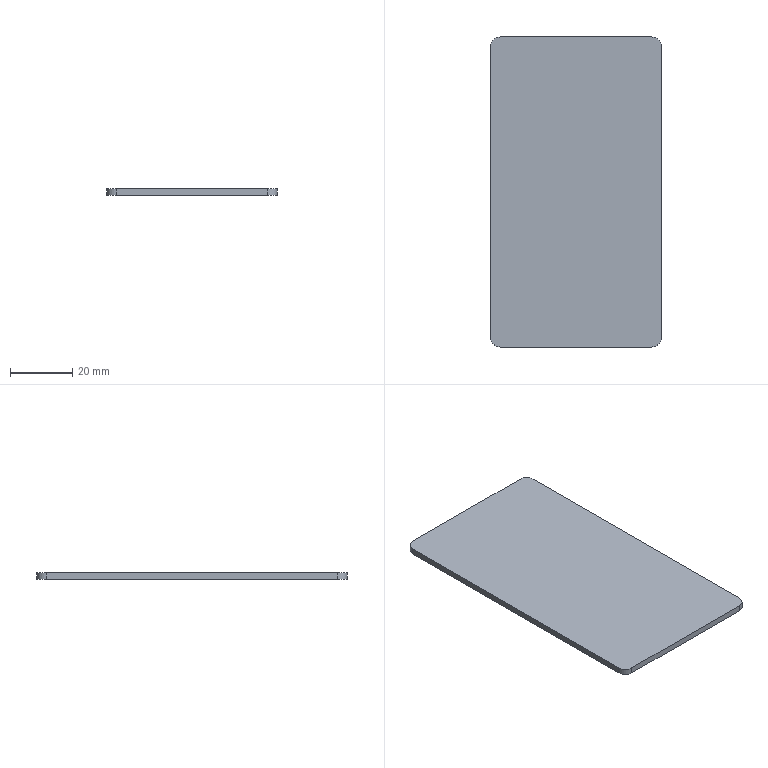Part | STEP file | E3-踢脚Plate支Plate | 1 solid | 10 faces | box 55 x 100 x 2 mm | volume 10985 mm3 | plane 6 | cylinder 4 | commonest cylinder face diameters 6 x4
STEP:
#1=CARTESIAN_POINT('',(0.,0.,0.));
#2=DIRECTION('',(0.,0.,1.));
#3=DIRECTION('',(1.,0.,0.));
#4=AXIS2_PLACEMENT_3D('',#1,#2,#3);
#5=CARTESIAN_POINT('',(27.5,-47.,-2.));
#6=VERTEX_POINT('',#5);
#7=CARTESIAN_POINT('',(27.5,47.,-2.));
#8=VERTEX_POINT('',#7);
#9=CARTESIAN_POINT('',(27.5,50.,-2.));
#10=DIRECTION('',(0.,1.,0.));
#11=VECTOR('',#10,1.);
#12=LINE('',#9,#11);
#13=CARTESIAN_POINT('',(27.5,50.,-2.));
#14=DIRECTION('',(-1.,0.,0.));
#15=DIRECTION('',(0.,0.,-1.));
#16=AXIS2_PLACEMENT_3D('',#13,#14,#15);
#17=PLANE('',#16);
#18=CARTESIAN_POINT('',(0.,0.));
#19=DIRECTION('',(0.,-1.));
#20=VECTOR('',#19,1.);
#21=LINE('',#18,#20);
#22=(GEOMETRIC_REPRESENTATION_CONTEXT(2)PARAMETRIC_REPRESENTATION_CONTEXT()REPRESENTATION_CONTEXT('',''));
#23=DEFINITIONAL_REPRESENTATION('',(#21),#22);
#24=PCURVE('',#17,#23);
#25=CARTESIAN_POINT('',(0.,0.,-2.));
#26=DIRECTION('',(0.,0.,-1.));
#27=DIRECTION('',(1.,0.,0.));
#28=AXIS2_PLACEMENT_3D('',#25,#26,#27);
#29=PLANE('',#28);
#30=CARTESIAN_POINT('',(27.5,-50.));
#31=DIRECTION('',(0.,-1.));
#32=VECTOR('',#31,1.);
#33=LINE('',#30,#32);
#34=(GEOMETRIC_REPRESENTATION_CONTEXT(2)PARAMETRIC_REPRESENTATION_CONTEXT()REPRESENTATION_CONTEXT('',''));
#35=DEFINITIONAL_REPRESENTATION('',(#33),#34);
#36=PCURVE('',#29,#35);
#37=SURFACE_CURVE('',#12,(#24,#36),.PCURVE_S1.);
#38=EDGE_CURVE('',#6,#8,#37,.T.);
#39=ORIENTED_EDGE('',*,*,#38,.T.);
#40=CARTESIAN_POINT('',(27.5,47.,0.));
#41=VERTEX_POINT('',#40);
#42=CARTESIAN_POINT('',(27.5,47.,-2.));
#43=DIRECTION('',(0.,0.,-1.));
#44=VECTOR('',#43,1.);
#45=LINE('',#42,#44);
#46=CARTESIAN_POINT('',(0.,3.));
#47=DIRECTION('',(1.,0.));
#48=VECTOR('',#47,1.);
#49=LINE('',#46,#48);
#50=(GEOMETRIC_REPRESENTATION_CONTEXT(2)PARAMETRIC_REPRESENTATION_CONTEXT()REPRESENTATION_CONTEXT('',''));
#51=DEFINITIONAL_REPRESENTATION('',(#49),#50);
#52=PCURVE('',#17,#51);
#53=CARTESIAN_POINT('',(24.5,47.,-2.));
#54=DIRECTION('',(0.,0.,1.));
#55=DIRECTION('',(-1.,0.,0.));
#56=AXIS2_PLACEMENT_3D('',#53,#54,#55);
#57=CYLINDRICAL_SURFACE('',#56,3.);
#58=CARTESIAN_POINT('',(3.142,0.));
#59=DIRECTION('',(0.,-1.));
#60=VECTOR('',#59,1.);
#61=LINE('',#58,#60);
#62=(GEOMETRIC_REPRESENTATION_CONTEXT(2)PARAMETRIC_REPRESENTATION_CONTEXT()REPRESENTATION_CONTEXT('',''));
#63=DEFINITIONAL_REPRESENTATION('',(#61),#62);
#64=PCURVE('',#57,#63);
#65=SURFACE_CURVE('',#45,(#52,#64),.PCURVE_S1.);
#66=EDGE_CURVE('',#41,#8,#65,.T.);
#67=ORIENTED_EDGE('',*,*,#66,.F.);
#68=CARTESIAN_POINT('',(27.5,-47.,0.));
#69=VERTEX_POINT('',#68);
#70=CARTESIAN_POINT('',(27.5,50.,0.));
#71=DIRECTION('',(0.,1.,0.));
#72=VECTOR('',#71,1.);
#73=LINE('',#70,#72);
#74=CARTESIAN_POINT('',(-2.,0.));
#75=DIRECTION('',(0.,-1.));
#76=VECTOR('',#75,1.);
#77=LINE('',#74,#76);
#78=(GEOMETRIC_REPRESENTATION_CONTEXT(2)PARAMETRIC_REPRESENTATION_CONTEXT()REPRESENTATION_CONTEXT('',''));
#79=DEFINITIONAL_REPRESENTATION('',(#77),#78);
#80=PCURVE('',#17,#79);
#81=CARTESIAN_POINT('',(0.,0.,0.));
#82=DIRECTION('',(0.,0.,-1.));
#83=DIRECTION('',(1.,0.,0.));
#84=AXIS2_PLACEMENT_3D('',#81,#82,#83);
#85=PLANE('',#84);
#86=CARTESIAN_POINT('',(27.5,-50.));
#87=DIRECTION('',(0.,-1.));
#88=VECTOR('',#87,1.);
#89=LINE('',#86,#88);
#90=(GEOMETRIC_REPRESENTATION_CONTEXT(2)PARAMETRIC_REPRESENTATION_CONTEXT()REPRESENTATION_CONTEXT('',''));
#91=DEFINITIONAL_REPRESENTATION('',(#89),#90);
#92=PCURVE('',#85,#91);
#93=SURFACE_CURVE('',#73,(#80,#92),.PCURVE_S1.);
#94=EDGE_CURVE('',#69,#41,#93,.T.);
#95=ORIENTED_EDGE('',*,*,#94,.F.);
#96=CARTESIAN_POINT('',(27.5,-47.,-2.));
#97=DIRECTION('',(0.,0.,1.));
#98=VECTOR('',#97,1.);
#99=LINE('',#96,#98);
#100=CARTESIAN_POINT('',(0.,97.));
#101=DIRECTION('',(-1.,0.));
#102=VECTOR('',#101,1.);
#103=LINE('',#100,#102);
#104=(GEOMETRIC_REPRESENTATION_CONTEXT(2)PARAMETRIC_REPRESENTATION_CONTEXT()REPRESENTATION_CONTEXT('',''));
#105=DEFINITIONAL_REPRESENTATION('',(#103),#104);
#106=PCURVE('',#17,#105);
#107=CARTESIAN_POINT('',(24.5,-47.,-2.));
#108=DIRECTION('',(0.,0.,1.));
#109=DIRECTION('',(-1.,0.,0.));
#110=AXIS2_PLACEMENT_3D('',#107,#108,#109);
#111=CYLINDRICAL_SURFACE('',#110,3.);
#112=CARTESIAN_POINT('',(3.142,0.));
#113=DIRECTION('',(0.,1.));
#114=VECTOR('',#113,1.);
#115=LINE('',#112,#114);
#116=(GEOMETRIC_REPRESENTATION_CONTEXT(2)PARAMETRIC_REPRESENTATION_CONTEXT()REPRESENTATION_CONTEXT('',''));
#117=DEFINITIONAL_REPRESENTATION('',(#115),#116);
#118=PCURVE('',#111,#117);
#119=SURFACE_CURVE('',#99,(#106,#118),.PCURVE_S1.);
#120=EDGE_CURVE('',#6,#69,#119,.T.);
#121=ORIENTED_EDGE('',*,*,#120,.F.);
#122=EDGE_LOOP('',(#39,#67,#95,#121));
#123=FACE_BOUND('',#122,.T.);
#124=ADVANCED_FACE('',(#123),#17,.F.);
#125=CARTESIAN_POINT('',(24.5,50.,-2.));
#126=VERTEX_POINT('',#125);
#127=CARTESIAN_POINT('',(-24.5,50.,-2.));
#128=VERTEX_POINT('',#127);
#129=CARTESIAN_POINT('',(-27.5,50.,-2.));
#130=DIRECTION('',(-1.,0.,0.));
#131=VECTOR('',#130,1.);
#132=LINE('',#129,#131);
#133=CARTESIAN_POINT('',(-27.5,50.,-2.));
#134=DIRECTION('',(0.,-1.,0.));
#135=DIRECTION('',(0.,0.,1.));
#136=AXIS2_PLACEMENT_3D('',#133,#134,#135);
#137=PLANE('',#136);
#138=CARTESIAN_POINT('',(0.,0.));
#139=DIRECTION('',(0.,1.));
#140=VECTOR('',#139,1.);
#141=LINE('',#138,#140);
#142=(GEOMETRIC_REPRESENTATION_CONTEXT(2)PARAMETRIC_REPRESENTATION_CONTEXT()REPRESENTATION_CONTEXT('',''));
#143=DEFINITIONAL_REPRESENTATION('',(#141),#142);
#144=PCURVE('',#137,#143);
#145=CARTESIAN_POINT('',(-27.5,-50.));
#146=DIRECTION('',(-1.,0.));
#147=VECTOR('',#146,1.);
#148=LINE('',#145,#147);
#149=(GEOMETRIC_REPRESENTATION_CONTEXT(2)PARAMETRIC_REPRESENTATION_CONTEXT()REPRESENTATION_CONTEXT('',''));
#150=DEFINITIONAL_REPRESENTATION('',(#148),#149);
#151=PCURVE('',#29,#150);
#152=SURFACE_CURVE('',#132,(#144,#151),.PCURVE_S1.);
#153=EDGE_CURVE('',#126,#128,#152,.T.);
#154=ORIENTED_EDGE('',*,*,#153,.T.);
#155=CARTESIAN_POINT('',(-24.5,50.,0.));
#156=VERTEX_POINT('',#155);
#157=CARTESIAN_POINT('',(-24.5,50.,-2.));
#158=DIRECTION('',(0.,0.,-1.));
#159=VECTOR('',#158,1.);
#160=LINE('',#157,#159);
#161=CARTESIAN_POINT('',(0.,-3.));
#162=DIRECTION('',(-1.,0.));
#163=VECTOR('',#162,1.);
#164=LINE('',#161,#163);
#165=(GEOMETRIC_REPRESENTATION_CONTEXT(2)PARAMETRIC_REPRESENTATION_CONTEXT()REPRESENTATION_CONTEXT('',''));
#166=DEFINITIONAL_REPRESENTATION('',(#164),#165);
#167=PCURVE('',#137,#166);
#168=CARTESIAN_POINT('',(-24.5,47.,-2.));
#169=DIRECTION('',(0.,0.,1.));
#170=DIRECTION('',(-1.,0.,0.));
#171=AXIS2_PLACEMENT_3D('',#168,#169,#170);
#172=CYLINDRICAL_SURFACE('',#171,3.);
#173=CARTESIAN_POINT('',(4.712,0.));
#174=DIRECTION('',(0.,-1.));
#175=VECTOR('',#174,1.);
#176=LINE('',#173,#175);
#177=(GEOMETRIC_REPRESENTATION_CONTEXT(2)PARAMETRIC_REPRESENTATION_CONTEXT()REPRESENTATION_CONTEXT('',''));
#178=DEFINITIONAL_REPRESENTATION('',(#176),#177);
#179=PCURVE('',#172,#178);
#180=SURFACE_CURVE('',#160,(#167,#179),.PCURVE_S1.);
#181=EDGE_CURVE('',#156,#128,#180,.T.);
#182=ORIENTED_EDGE('',*,*,#181,.F.);
#183=CARTESIAN_POINT('',(24.5,50.,0.));
#184=VERTEX_POINT('',#183);
#185=CARTESIAN_POINT('',(-27.5,50.,0.));
#186=DIRECTION('',(-1.,0.,0.));
#187=VECTOR('',#186,1.);
#188=LINE('',#185,#187);
#189=CARTESIAN_POINT('',(2.,0.));
#190=DIRECTION('',(0.,1.));
#191=VECTOR('',#190,1.);
#192=LINE('',#189,#191);
#193=(GEOMETRIC_REPRESENTATION_CONTEXT(2)PARAMETRIC_REPRESENTATION_CONTEXT()REPRESENTATION_CONTEXT('',''));
#194=DEFINITIONAL_REPRESENTATION('',(#192),#193);
#195=PCURVE('',#137,#194);
#196=CARTESIAN_POINT('',(-27.5,-50.));
#197=DIRECTION('',(-1.,0.));
#198=VECTOR('',#197,1.);
#199=LINE('',#196,#198);
#200=(GEOMETRIC_REPRESENTATION_CONTEXT(2)PARAMETRIC_REPRESENTATION_CONTEXT()REPRESENTATION_CONTEXT('',''));
#201=DEFINITIONAL_REPRESENTATION('',(#199),#200);
#202=PCURVE('',#85,#201);
#203=SURFACE_CURVE('',#188,(#195,#202),.PCURVE_S1.);
#204=EDGE_CURVE('',#184,#156,#203,.T.);
#205=ORIENTED_EDGE('',*,*,#204,.F.);
#206=CARTESIAN_POINT('',(24.5,50.,-2.));
#207=DIRECTION('',(0.,0.,1.));
#208=VECTOR('',#207,1.);
#209=LINE('',#206,#208);
#210=CARTESIAN_POINT('',(0.,-52.));
#211=DIRECTION('',(1.,0.));
#212=VECTOR('',#211,1.);
#213=LINE('',#210,#212);
#214=(GEOMETRIC_REPRESENTATION_CONTEXT(2)PARAMETRIC_REPRESENTATION_CONTEXT()REPRESENTATION_CONTEXT('',''));
#215=DEFINITIONAL_REPRESENTATION('',(#213),#214);
#216=PCURVE('',#137,#215);
#217=CARTESIAN_POINT('',(4.712,0.));
#218=DIRECTION('',(0.,1.));
#219=VECTOR('',#218,1.);
#220=LINE('',#217,#219);
#221=(GEOMETRIC_REPRESENTATION_CONTEXT(2)PARAMETRIC_REPRESENTATION_CONTEXT()REPRESENTATION_CONTEXT('',''));
#222=DEFINITIONAL_REPRESENTATION('',(#220),#221);
#223=PCURVE('',#57,#222);
#224=SURFACE_CURVE('',#209,(#216,#223),.PCURVE_S1.);
#225=EDGE_CURVE('',#126,#184,#224,.T.);
#226=ORIENTED_EDGE('',*,*,#225,.F.);
#227=EDGE_LOOP('',(#154,#182,#205,#226));
#228=FACE_BOUND('',#227,.T.);
#229=ADVANCED_FACE('',(#228),#137,.F.);
#230=CARTESIAN_POINT('',(-27.5,47.,0.));
#231=VERTEX_POINT('',#230);
#232=CARTESIAN_POINT('',(-27.5,-47.,0.));
#233=VERTEX_POINT('',#232);
#234=CARTESIAN_POINT('',(-27.5,50.,0.));
#235=DIRECTION('',(0.,-1.,0.));
#236=VECTOR('',#235,1.);
#237=LINE('',#234,#236);
#238=CARTESIAN_POINT('',(-27.5,50.,-2.));
#239=DIRECTION('',(1.,0.,0.));
#240=DIRECTION('',(0.,0.,1.));
#241=AXIS2_PLACEMENT_3D('',#238,#239,#240);
#242=PLANE('',#241);
#243=CARTESIAN_POINT('',(2.,0.));
#244=DIRECTION('',(0.,1.));
#245=VECTOR('',#244,1.);
#246=LINE('',#243,#245);
#247=(GEOMETRIC_REPRESENTATION_CONTEXT(2)PARAMETRIC_REPRESENTATION_CONTEXT()REPRESENTATION_CONTEXT('',''));
#248=DEFINITIONAL_REPRESENTATION('',(#246),#247);
#249=PCURVE('',#242,#248);
#250=CARTESIAN_POINT('',(-27.5,-50.));
#251=DIRECTION('',(0.,1.));
#252=VECTOR('',#251,1.);
#253=LINE('',#250,#252);
#254=(GEOMETRIC_REPRESENTATION_CONTEXT(2)PARAMETRIC_REPRESENTATION_CONTEXT()REPRESENTATION_CONTEXT('',''));
#255=DEFINITIONAL_REPRESENTATION('',(#253),#254);
#256=PCURVE('',#85,#255);
#257=SURFACE_CURVE('',#237,(#249,#256),.PCURVE_S1.);
#258=EDGE_CURVE('',#231,#233,#257,.T.);
#259=ORIENTED_EDGE('',*,*,#258,.F.);
#260=CARTESIAN_POINT('',(-27.5,47.,-2.));
#261=VERTEX_POINT('',#260);
#262=CARTESIAN_POINT('',(-27.5,47.,-2.));
#263=DIRECTION('',(0.,0.,1.));
#264=VECTOR('',#263,1.);
#265=LINE('',#262,#264);
#266=CARTESIAN_POINT('',(0.,3.));
#267=DIRECTION('',(1.,0.));
#268=VECTOR('',#267,1.);
#269=LINE('',#266,#268);
#270=(GEOMETRIC_REPRESENTATION_CONTEXT(2)PARAMETRIC_REPRESENTATION_CONTEXT()REPRESENTATION_CONTEXT('',''));
#271=DEFINITIONAL_REPRESENTATION('',(#269),#270);
#272=PCURVE('',#242,#271);
#273=CARTESIAN_POINT('',(6.283,0.));
#274=DIRECTION('',(0.,1.));
#275=VECTOR('',#274,1.);
#276=LINE('',#273,#275);
#277=(GEOMETRIC_REPRESENTATION_CONTEXT(2)PARAMETRIC_REPRESENTATION_CONTEXT()REPRESENTATION_CONTEXT('',''));
#278=DEFINITIONAL_REPRESENTATION('',(#276),#277);
#279=PCURVE('',#172,#278);
#280=SURFACE_CURVE('',#265,(#272,#279),.PCURVE_S1.);
#281=EDGE_CURVE('',#261,#231,#280,.T.);
#282=ORIENTED_EDGE('',*,*,#281,.F.);
#283=CARTESIAN_POINT('',(-27.5,-47.,-2.));
#284=VERTEX_POINT('',#283);
#285=CARTESIAN_POINT('',(-27.5,50.,-2.));
#286=DIRECTION('',(0.,-1.,0.));
#287=VECTOR('',#286,1.);
#288=LINE('',#285,#287);
#289=CARTESIAN_POINT('',(0.,0.));
#290=DIRECTION('',(0.,1.));
#291=VECTOR('',#290,1.);
#292=LINE('',#289,#291);
#293=(GEOMETRIC_REPRESENTATION_CONTEXT(2)PARAMETRIC_REPRESENTATION_CONTEXT()REPRESENTATION_CONTEXT('',''));
#294=DEFINITIONAL_REPRESENTATION('',(#292),#293);
#295=PCURVE('',#242,#294);
#296=CARTESIAN_POINT('',(-27.5,-50.));
#297=DIRECTION('',(0.,1.));
#298=VECTOR('',#297,1.);
#299=LINE('',#296,#298);
#300=(GEOMETRIC_REPRESENTATION_CONTEXT(2)PARAMETRIC_REPRESENTATION_CONTEXT()REPRESENTATION_CONTEXT('',''));
#301=DEFINITIONAL_REPRESENTATION('',(#299),#300);
#302=PCURVE('',#29,#301);
#303=SURFACE_CURVE('',#288,(#295,#302),.PCURVE_S1.);
#304=EDGE_CURVE('',#261,#284,#303,.T.);
#305=ORIENTED_EDGE('',*,*,#304,.T.);
#306=CARTESIAN_POINT('',(-27.5,-47.,-2.));
#307=DIRECTION('',(0.,0.,-1.));
#308=VECTOR('',#307,1.);
#309=LINE('',#306,#308);
#310=CARTESIAN_POINT('',(0.,97.));
#311=DIRECTION('',(-1.,0.));
#312=VECTOR('',#311,1.);
#313=LINE('',#310,#312);
#314=(GEOMETRIC_REPRESENTATION_CONTEXT(2)PARAMETRIC_REPRESENTATION_CONTEXT()REPRESENTATION_CONTEXT('',''));
#315=DEFINITIONAL_REPRESENTATION('',(#313),#314);
#316=PCURVE('',#242,#315);
#317=CARTESIAN_POINT('',(-24.5,-47.,-2.));
#318=DIRECTION('',(0.,0.,1.));
#319=DIRECTION('',(-1.,0.,0.));
#320=AXIS2_PLACEMENT_3D('',#317,#318,#319);
#321=CYLINDRICAL_SURFACE('',#320,3.);
#322=CARTESIAN_POINT('',(0.,0.));
#323=DIRECTION('',(0.,-1.));
#324=VECTOR('',#323,1.);
#325=LINE('',#322,#324);
#326=(GEOMETRIC_REPRESENTATION_CONTEXT(2)PARAMETRIC_REPRESENTATION_CONTEXT()REPRESENTATION_CONTEXT('',''));
#327=DEFINITIONAL_REPRESENTATION('',(#325),#326);
#328=PCURVE('',#321,#327);
#329=SURFACE_CURVE('',#309,(#316,#328),.PCURVE_S1.);
#330=EDGE_CURVE('',#233,#284,#329,.T.);
#331=ORIENTED_EDGE('',*,*,#330,.F.);
#332=EDGE_LOOP('',(#259,#282,#305,#331));
#333=FACE_BOUND('',#332,.T.);
#334=ADVANCED_FACE('',(#333),#242,.F.);
#335=CARTESIAN_POINT('',(-24.5,-50.,0.));
#336=VERTEX_POINT('',#335);
#337=CARTESIAN_POINT('',(24.5,-50.,0.));
#338=VERTEX_POINT('',#337);
#339=CARTESIAN_POINT('',(-27.5,-50.,0.));
#340=DIRECTION('',(1.,0.,0.));
#341=VECTOR('',#340,1.);
#342=LINE('',#339,#341);
#343=CARTESIAN_POINT('',(-27.5,-50.,-2.));
#344=DIRECTION('',(0.,1.,0.));
#345=DIRECTION('',(0.,0.,-1.));
#346=AXIS2_PLACEMENT_3D('',#343,#344,#345);
#347=PLANE('',#346);
#348=CARTESIAN_POINT('',(-2.,0.));
#349=DIRECTION('',(0.,-1.));
#350=VECTOR('',#349,1.);
#351=LINE('',#348,#350);
#352=(GEOMETRIC_REPRESENTATION_CONTEXT(2)PARAMETRIC_REPRESENTATION_CONTEXT()REPRESENTATION_CONTEXT('',''));
#353=DEFINITIONAL_REPRESENTATION('',(#351),#352);
#354=PCURVE('',#347,#353);
#355=CARTESIAN_POINT('',(-27.5,50.));
#356=DIRECTION('',(1.,0.));
#357=VECTOR('',#356,1.);
#358=LINE('',#355,#357);
#359=(GEOMETRIC_REPRESENTATION_CONTEXT(2)PARAMETRIC_REPRESENTATION_CONTEXT()REPRESENTATION_CONTEXT('',''));
#360=DEFINITIONAL_REPRESENTATION('',(#358),#359);
#361=PCURVE('',#85,#360);
#362=SURFACE_CURVE('',#342,(#354,#361),.PCURVE_S1.);
#363=EDGE_CURVE('',#336,#338,#362,.T.);
#364=ORIENTED_EDGE('',*,*,#363,.F.);
#365=CARTESIAN_POINT('',(-24.5,-50.,-2.));
#366=VERTEX_POINT('',#365);
#367=CARTESIAN_POINT('',(-24.5,-50.,-2.));
#368=DIRECTION('',(0.,0.,1.));
#369=VECTOR('',#368,1.);
#370=LINE('',#367,#369);
#371=CARTESIAN_POINT('',(0.,-3.));
#372=DIRECTION('',(-1.,0.));
#373=VECTOR('',#372,1.);
#374=LINE('',#371,#373);
#375=(GEOMETRIC_REPRESENTATION_CONTEXT(2)PARAMETRIC_REPRESENTATION_CONTEXT()REPRESENTATION_CONTEXT('',''));
#376=DEFINITIONAL_REPRESENTATION('',(#374),#375);
#377=PCURVE('',#347,#376);
#378=CARTESIAN_POINT('',(1.571,0.));
#379=DIRECTION('',(0.,1.));
#380=VECTOR('',#379,1.);
#381=LINE('',#378,#380);
#382=(GEOMETRIC_REPRESENTATION_CONTEXT(2)PARAMETRIC_REPRESENTATION_CONTEXT()REPRESENTATION_CONTEXT('',''));
#383=DEFINITIONAL_REPRESENTATION('',(#381),#382);
#384=PCURVE('',#321,#383);
#385=SURFACE_CURVE('',#370,(#377,#384),.PCURVE_S1.);
#386=EDGE_CURVE('',#366,#336,#385,.T.);
#387=ORIENTED_EDGE('',*,*,#386,.F.);
#388=CARTESIAN_POINT('',(24.5,-50.,-2.));
#389=VERTEX_POINT('',#388);
#390=CARTESIAN_POINT('',(-27.5,-50.,-2.));
#391=DIRECTION('',(1.,0.,0.));
#392=VECTOR('',#391,1.);
#393=LINE('',#390,#392);
#394=CARTESIAN_POINT('',(0.,0.));
#395=DIRECTION('',(0.,-1.));
#396=VECTOR('',#395,1.);
#397=LINE('',#394,#396);
#398=(GEOMETRIC_REPRESENTATION_CONTEXT(2)PARAMETRIC_REPRESENTATION_CONTEXT()REPRESENTATION_CONTEXT('',''));
#399=DEFINITIONAL_REPRESENTATION('',(#397),#398);
#400=PCURVE('',#347,#399);
#401=CARTESIAN_POINT('',(-27.5,50.));
#402=DIRECTION('',(1.,0.));
#403=VECTOR('',#402,1.);
#404=LINE('',#401,#403);
#405=(GEOMETRIC_REPRESENTATION_CONTEXT(2)PARAMETRIC_REPRESENTATION_CONTEXT()REPRESENTATION_CONTEXT('',''));
#406=DEFINITIONAL_REPRESENTATION('',(#404),#405);
#407=PCURVE('',#29,#406);
#408=SURFACE_CURVE('',#393,(#400,#407),.PCURVE_S1.);
#409=EDGE_CURVE('',#366,#389,#408,.T.);
#410=ORIENTED_EDGE('',*,*,#409,.T.);
#411=CARTESIAN_POINT('',(24.5,-50.,-2.));
#412=DIRECTION('',(0.,0.,-1.));
#413=VECTOR('',#412,1.);
#414=LINE('',#411,#413);
#415=CARTESIAN_POINT('',(0.,-52.));
#416=DIRECTION('',(1.,0.));
#417=VECTOR('',#416,1.);
#418=LINE('',#415,#417);
#419=(GEOMETRIC_REPRESENTATION_CONTEXT(2)PARAMETRIC_REPRESENTATION_CONTEXT()REPRESENTATION_CONTEXT('',''));
#420=DEFINITIONAL_REPRESENTATION('',(#418),#419);
#421=PCURVE('',#347,#420);
#422=CARTESIAN_POINT('',(1.571,0.));
#423=DIRECTION('',(0.,-1.));
#424=VECTOR('',#423,1.);
#425=LINE('',#422,#424);
#426=(GEOMETRIC_REPRESENTATION_CONTEXT(2)PARAMETRIC_REPRESENTATION_CONTEXT()REPRESENTATION_CONTEXT('',''));
#427=DEFINITIONAL_REPRESENTATION('',(#425),#426);
#428=PCURVE('',#111,#427);
#429=SURFACE_CURVE('',#414,(#421,#428),.PCURVE_S1.);
#430=EDGE_CURVE('',#338,#389,#429,.T.);
#431=ORIENTED_EDGE('',*,*,#430,.F.);
#432=EDGE_LOOP('',(#364,#387,#410,#431));
#433=FACE_BOUND('',#432,.T.);
#434=ADVANCED_FACE('',(#433),#347,.F.);
#435=ORIENTED_EDGE('',*,*,#409,.F.);
#436=CARTESIAN_POINT('',(-24.5,-47.,-2.));
#437=DIRECTION('',(0.,0.,1.));
#438=DIRECTION('',(1.,0.,0.));
#439=AXIS2_PLACEMENT_3D('',#436,#437,#438);
#440=CIRCLE('',#439,3.);
#441=CARTESIAN_POINT('',(-21.5,47.));
#442=CARTESIAN_POINT('',(-21.5,41.804));
#443=CARTESIAN_POINT('',(-26.,44.402));
#444=CARTESIAN_POINT('',(-30.5,47.));
#445=CARTESIAN_POINT('',(-26.,49.598));
#446=CARTESIAN_POINT('',(-21.5,52.196));
#447=CARTESIAN_POINT('',(-21.5,47.));
#448=(BOUNDED_CURVE()B_SPLINE_CURVE(2,(#441,#442,#443,#444,#445,#446,#447),.UNSPECIFIED.,.T.,.F.)B_SPLINE_CURVE_WITH_KNOTS((1,2,2,2,2,1),(-2.094,0.,2.094,4.189,6.283,8.378),.UNSPECIFIED.)CURVE()GEOMETRIC_REPRESENTATION_ITEM()RATIONAL_B_SPLINE_CURVE((1.,0.5,1.,0.5,1.,0.5,1.))REPRESENTATION_ITEM(''));
#449=(GEOMETRIC_REPRESENTATION_CONTEXT(2)PARAMETRIC_REPRESENTATION_CONTEXT()REPRESENTATION_CONTEXT('',''));
#450=DEFINITIONAL_REPRESENTATION('',(#448),#449);
#451=PCURVE('',#29,#450);
#452=CARTESIAN_POINT('',(-3.142,0.));
#453=DIRECTION('',(1.,0.));
#454=VECTOR('',#453,1.);
#455=LINE('',#452,#454);
#456=(GEOMETRIC_REPRESENTATION_CONTEXT(2)PARAMETRIC_REPRESENTATION_CONTEXT()REPRESENTATION_CONTEXT('',''));
#457=DEFINITIONAL_REPRESENTATION('',(#455),#456);
#458=PCURVE('',#321,#457);
#459=SURFACE_CURVE('',#440,(#451,#458),.PCURVE_S1.);
#460=EDGE_CURVE('',#284,#366,#459,.T.);
#461=ORIENTED_EDGE('',*,*,#460,.F.);
#462=ORIENTED_EDGE('',*,*,#304,.F.);
#463=CARTESIAN_POINT('',(-24.5,47.,-2.));
#464=DIRECTION('',(0.,0.,1.));
#465=DIRECTION('',(1.,0.,0.));
#466=AXIS2_PLACEMENT_3D('',#463,#464,#465);
#467=CIRCLE('',#466,3.);
#468=CARTESIAN_POINT('',(-21.5,-47.));
#469=CARTESIAN_POINT('',(-21.5,-52.196));
#470=CARTESIAN_POINT('',(-26.,-49.598));
#471=CARTESIAN_POINT('',(-30.5,-47.));
#472=CARTESIAN_POINT('',(-26.,-44.402));
#473=CARTESIAN_POINT('',(-21.5,-41.804));
#474=CARTESIAN_POINT('',(-21.5,-47.));
#475=(BOUNDED_CURVE()B_SPLINE_CURVE(2,(#468,#469,#470,#471,#472,#473,#474),.UNSPECIFIED.,.T.,.F.)B_SPLINE_CURVE_WITH_KNOTS((1,2,2,2,2,1),(-2.094,0.,2.094,4.189,6.283,8.378),.UNSPECIFIED.)CURVE()GEOMETRIC_REPRESENTATION_ITEM()RATIONAL_B_SPLINE_CURVE((1.,0.5,1.,0.5,1.,0.5,1.))REPRESENTATION_ITEM(''));
#476=(GEOMETRIC_REPRESENTATION_CONTEXT(2)PARAMETRIC_REPRESENTATION_CONTEXT()REPRESENTATION_CONTEXT('',''));
#477=DEFINITIONAL_REPRESENTATION('',(#475),#476);
#478=PCURVE('',#29,#477);
#479=CARTESIAN_POINT('',(3.142,0.));
#480=DIRECTION('',(1.,0.));
#481=VECTOR('',#480,1.);
#482=LINE('',#479,#481);
#483=(GEOMETRIC_REPRESENTATION_CONTEXT(2)PARAMETRIC_REPRESENTATION_CONTEXT()REPRESENTATION_CONTEXT('',''));
#484=DEFINITIONAL_REPRESENTATION('',(#482),#483);
#485=PCURVE('',#172,#484);
#486=SURFACE_CURVE('',#467,(#478,#485),.PCURVE_S1.);
#487=EDGE_CURVE('',#128,#261,#486,.T.);
#488=ORIENTED_EDGE('',*,*,#487,.F.);
#489=ORIENTED_EDGE('',*,*,#153,.F.);
#490=CARTESIAN_POINT('',(24.5,47.,-2.));
#491=DIRECTION('',(0.,0.,1.));
#492=DIRECTION('',(1.,0.,0.));
#493=AXIS2_PLACEMENT_3D('',#490,#491,#492);
#494=CIRCLE('',#493,3.);
#495=CARTESIAN_POINT('',(27.5,-47.));
#496=CARTESIAN_POINT('',(27.5,-52.196));
#497=CARTESIAN_POINT('',(23.,-49.598));
#498=CARTESIAN_POINT('',(18.5,-47.));
#499=CARTESIAN_POINT('',(23.,-44.402));
#500=CARTESIAN_POINT('',(27.5,-41.804));
#501=CARTESIAN_POINT('',(27.5,-47.));
#502=(BOUNDED_CURVE()B_SPLINE_CURVE(2,(#495,#496,#497,#498,#499,#500,#501),.UNSPECIFIED.,.T.,.F.)B_SPLINE_CURVE_WITH_KNOTS((1,2,2,2,2,1),(-2.094,0.,2.094,4.189,6.283,8.378),.UNSPECIFIED.)CURVE()GEOMETRIC_REPRESENTATION_ITEM()RATIONAL_B_SPLINE_CURVE((1.,0.5,1.,0.5,1.,0.5,1.))REPRESENTATION_ITEM(''));
#503=(GEOMETRIC_REPRESENTATION_CONTEXT(2)PARAMETRIC_REPRESENTATION_CONTEXT()REPRESENTATION_CONTEXT('',''));
#504=DEFINITIONAL_REPRESENTATION('',(#502),#503);
#505=PCURVE('',#29,#504);
#506=CARTESIAN_POINT('',(3.142,0.));
#507=DIRECTION('',(1.,0.));
#508=VECTOR('',#507,1.);
#509=LINE('',#506,#508);
#510=(GEOMETRIC_REPRESENTATION_CONTEXT(2)PARAMETRIC_REPRESENTATION_CONTEXT()REPRESENTATION_CONTEXT('',''));
#511=DEFINITIONAL_REPRESENTATION('',(#509),#510);
#512=PCURVE('',#57,#511);
#513=SURFACE_CURVE('',#494,(#505,#512),.PCURVE_S1.);
#514=EDGE_CURVE('',#8,#126,#513,.T.);
#515=ORIENTED_EDGE('',*,*,#514,.F.);
#516=ORIENTED_EDGE('',*,*,#38,.F.);
#517=CARTESIAN_POINT('',(24.5,-47.,-2.));
#518=DIRECTION('',(0.,0.,1.));
#519=DIRECTION('',(1.,0.,0.));
#520=AXIS2_PLACEMENT_3D('',#517,#518,#519);
#521=CIRCLE('',#520,3.);
#522=CARTESIAN_POINT('',(27.5,47.));
#523=CARTESIAN_POINT('',(27.5,41.804));
#524=CARTESIAN_POINT('',(23.,44.402));
#525=CARTESIAN_POINT('',(18.5,47.));
#526=CARTESIAN_POINT('',(23.,49.598));
#527=CARTESIAN_POINT('',(27.5,52.196));
#528=CARTESIAN_POINT('',(27.5,47.));
#529=(BOUNDED_CURVE()B_SPLINE_CURVE(2,(#522,#523,#524,#525,#526,#527,#528),.UNSPECIFIED.,.T.,.F.)B_SPLINE_CURVE_WITH_KNOTS((1,2,2,2,2,1),(-2.094,0.,2.094,4.189,6.283,8.378),.UNSPECIFIED.)CURVE()GEOMETRIC_REPRESENTATION_ITEM()RATIONAL_B_SPLINE_CURVE((1.,0.5,1.,0.5,1.,0.5,1.))REPRESENTATION_ITEM(''));
#530=(GEOMETRIC_REPRESENTATION_CONTEXT(2)PARAMETRIC_REPRESENTATION_CONTEXT()REPRESENTATION_CONTEXT('',''));
#531=DEFINITIONAL_REPRESENTATION('',(#529),#530);
#532=PCURVE('',#29,#531);
#533=CARTESIAN_POINT('',(-3.142,0.));
#534=DIRECTION('',(1.,0.));
#535=VECTOR('',#534,1.);
#536=LINE('',#533,#535);
#537=(GEOMETRIC_REPRESENTATION_CONTEXT(2)PARAMETRIC_REPRESENTATION_CONTEXT()REPRESENTATION_CONTEXT('',''));
#538=DEFINITIONAL_REPRESENTATION('',(#536),#537);
#539=PCURVE('',#111,#538);
#540=SURFACE_CURVE('',#521,(#532,#539),.PCURVE_S1.);
#541=EDGE_CURVE('',#389,#6,#540,.T.);
#542=ORIENTED_EDGE('',*,*,#541,.F.);
#543=EDGE_LOOP('',(#435,#461,#462,#488,#489,#515,#516,#542));
#544=FACE_BOUND('',#543,.T.);
#545=ADVANCED_FACE('',(#544),#29,.T.);
#546=ORIENTED_EDGE('',*,*,#94,.T.);
#547=CARTESIAN_POINT('',(24.5,47.,0.));
#548=DIRECTION('',(0.,0.,-1.));
#549=DIRECTION('',(1.,0.,0.));
#550=AXIS2_PLACEMENT_3D('',#547,#548,#549);
#551=CIRCLE('',#550,3.);
#552=CARTESIAN_POINT('',(24.5,-47.));
#553=DIRECTION('',(1.,0.));
#554=AXIS2_PLACEMENT_2D('',#552,#553);
#555=CIRCLE('',#554,3.);
#556=(GEOMETRIC_REPRESENTATION_CONTEXT(2)PARAMETRIC_REPRESENTATION_CONTEXT()REPRESENTATION_CONTEXT('',''));
#557=DEFINITIONAL_REPRESENTATION('',(#555),#556);
#558=PCURVE('',#85,#557);
#559=CARTESIAN_POINT('',(9.425,2.));
#560=DIRECTION('',(-1.,0.));
#561=VECTOR('',#560,1.);
#562=LINE('',#559,#561);
#563=(GEOMETRIC_REPRESENTATION_CONTEXT(2)PARAMETRIC_REPRESENTATION_CONTEXT()REPRESENTATION_CONTEXT('',''));
#564=DEFINITIONAL_REPRESENTATION('',(#562),#563);
#565=PCURVE('',#57,#564);
#566=SURFACE_CURVE('',#551,(#558,#565),.PCURVE_S1.);
#567=EDGE_CURVE('',#184,#41,#566,.T.);
#568=ORIENTED_EDGE('',*,*,#567,.F.);
#569=ORIENTED_EDGE('',*,*,#204,.T.);
#570=CARTESIAN_POINT('',(-24.5,47.,0.));
#571=DIRECTION('',(0.,0.,-1.));
#572=DIRECTION('',(1.,0.,0.));
#573=AXIS2_PLACEMENT_3D('',#570,#571,#572);
#574=CIRCLE('',#573,3.);
#575=CARTESIAN_POINT('',(-24.5,-47.));
#576=DIRECTION('',(1.,0.));
#577=AXIS2_PLACEMENT_2D('',#575,#576);
#578=CIRCLE('',#577,3.);
#579=(GEOMETRIC_REPRESENTATION_CONTEXT(2)PARAMETRIC_REPRESENTATION_CONTEXT()REPRESENTATION_CONTEXT('',''));
#580=DEFINITIONAL_REPRESENTATION('',(#578),#579);
#581=PCURVE('',#85,#580);
#582=CARTESIAN_POINT('',(9.425,2.));
#583=DIRECTION('',(-1.,0.));
#584=VECTOR('',#583,1.);
#585=LINE('',#582,#584);
#586=(GEOMETRIC_REPRESENTATION_CONTEXT(2)PARAMETRIC_REPRESENTATION_CONTEXT()REPRESENTATION_CONTEXT('',''));
#587=DEFINITIONAL_REPRESENTATION('',(#585),#586);
#588=PCURVE('',#172,#587);
#589=SURFACE_CURVE('',#574,(#581,#588),.PCURVE_S1.);
#590=EDGE_CURVE('',#231,#156,#589,.T.);
#591=ORIENTED_EDGE('',*,*,#590,.F.);
#592=ORIENTED_EDGE('',*,*,#258,.T.);
#593=CARTESIAN_POINT('',(-24.5,-47.,0.));
#594=DIRECTION('',(0.,0.,-1.));
#595=DIRECTION('',(1.,0.,0.));
#596=AXIS2_PLACEMENT_3D('',#593,#594,#595);
#597=CIRCLE('',#596,3.);
#598=CARTESIAN_POINT('',(-24.5,47.));
#599=DIRECTION('',(1.,0.));
#600=AXIS2_PLACEMENT_2D('',#598,#599);
#601=CIRCLE('',#600,3.);
#602=(GEOMETRIC_REPRESENTATION_CONTEXT(2)PARAMETRIC_REPRESENTATION_CONTEXT()REPRESENTATION_CONTEXT('',''));
#603=DEFINITIONAL_REPRESENTATION('',(#601),#602);
#604=PCURVE('',#85,#603);
#605=CARTESIAN_POINT('',(3.142,2.));
#606=DIRECTION('',(-1.,0.));
#607=VECTOR('',#606,1.);
#608=LINE('',#605,#607);
#609=(GEOMETRIC_REPRESENTATION_CONTEXT(2)PARAMETRIC_REPRESENTATION_CONTEXT()REPRESENTATION_CONTEXT('',''));
#610=DEFINITIONAL_REPRESENTATION('',(#608),#609);
#611=PCURVE('',#321,#610);
#612=SURFACE_CURVE('',#597,(#604,#611),.PCURVE_S1.);
#613=EDGE_CURVE('',#336,#233,#612,.T.);
#614=ORIENTED_EDGE('',*,*,#613,.F.);
#615=ORIENTED_EDGE('',*,*,#363,.T.);
#616=CARTESIAN_POINT('',(24.5,-47.,0.));
#617=DIRECTION('',(0.,0.,-1.));
#618=DIRECTION('',(1.,0.,0.));
#619=AXIS2_PLACEMENT_3D('',#616,#617,#618);
#620=CIRCLE('',#619,3.);
#621=CARTESIAN_POINT('',(24.5,47.));
#622=DIRECTION('',(1.,0.));
#623=AXIS2_PLACEMENT_2D('',#621,#622);
#624=CIRCLE('',#623,3.);
#625=(GEOMETRIC_REPRESENTATION_CONTEXT(2)PARAMETRIC_REPRESENTATION_CONTEXT()REPRESENTATION_CONTEXT('',''));
#626=DEFINITIONAL_REPRESENTATION('',(#624),#625);
#627=PCURVE('',#85,#626);
#628=CARTESIAN_POINT('',(3.142,2.));
#629=DIRECTION('',(-1.,0.));
#630=VECTOR('',#629,1.);
#631=LINE('',#628,#630);
#632=(GEOMETRIC_REPRESENTATION_CONTEXT(2)PARAMETRIC_REPRESENTATION_CONTEXT()REPRESENTATION_CONTEXT('',''));
#633=DEFINITIONAL_REPRESENTATION('',(#631),#632);
#634=PCURVE('',#111,#633);
#635=SURFACE_CURVE('',#620,(#627,#634),.PCURVE_S1.);
#636=EDGE_CURVE('',#69,#338,#635,.T.);
#637=ORIENTED_EDGE('',*,*,#636,.F.);
#638=EDGE_LOOP('',(#546,#568,#569,#591,#592,#614,#615,#637));
#639=FACE_BOUND('',#638,.T.);
#640=ADVANCED_FACE('',(#639),#85,.F.);
#641=ORIENTED_EDGE('',*,*,#541,.T.);
#642=ORIENTED_EDGE('',*,*,#120,.T.);
#643=ORIENTED_EDGE('',*,*,#636,.T.);
#644=ORIENTED_EDGE('',*,*,#430,.T.);
#645=EDGE_LOOP('',(#641,#642,#643,#644));
#646=FACE_BOUND('',#645,.T.);
#647=ADVANCED_FACE('',(#646),#111,.T.);
#648=ORIENTED_EDGE('',*,*,#460,.T.);
#649=ORIENTED_EDGE('',*,*,#386,.T.);
#650=ORIENTED_EDGE('',*,*,#613,.T.);
#651=ORIENTED_EDGE('',*,*,#330,.T.);
#652=EDGE_LOOP('',(#648,#649,#650,#651));
#653=FACE_BOUND('',#652,.T.);
#654=ADVANCED_FACE('',(#653),#321,.T.);
#655=ORIENTED_EDGE('',*,*,#514,.T.);
#656=ORIENTED_EDGE('',*,*,#225,.T.);
#657=ORIENTED_EDGE('',*,*,#567,.T.);
#658=ORIENTED_EDGE('',*,*,#66,.T.);
#659=EDGE_LOOP('',(#655,#656,#657,#658));
#660=FACE_BOUND('',#659,.T.);
#661=ADVANCED_FACE('',(#660),#57,.T.);
#662=ORIENTED_EDGE('',*,*,#487,.T.);
#663=ORIENTED_EDGE('',*,*,#281,.T.);
#664=ORIENTED_EDGE('',*,*,#590,.T.);
#665=ORIENTED_EDGE('',*,*,#181,.T.);
#666=EDGE_LOOP('',(#662,#663,#664,#665));
#667=FACE_BOUND('',#666,.T.);
#668=ADVANCED_FACE('',(#667),#172,.T.);
#669=CLOSED_SHELL('',(#124,#229,#334,#434,#545,#640,#647,#654,#661,#668));
#670=MANIFOLD_SOLID_BREP('',#669);
#671=(LENGTH_UNIT()NAMED_UNIT(*)SI_UNIT(.MILLI.,.METRE.));
#672=UNCERTAINTY_MEASURE_WITH_UNIT(LENGTH_MEASURE(0.0000001),#671,'','');
#673=(NAMED_UNIT(*)PLANE_ANGLE_UNIT()SI_UNIT($,.RADIAN.));
#674=(NAMED_UNIT(*)SI_UNIT($,.STERADIAN.)SOLID_ANGLE_UNIT());
#675=(GEOMETRIC_REPRESENTATION_CONTEXT(3)GLOBAL_UNCERTAINTY_ASSIGNED_CONTEXT((#672))GLOBAL_UNIT_ASSIGNED_CONTEXT((#671,#673,#674))REPRESENTATION_CONTEXT('',''));
#676=ADVANCED_BREP_SHAPE_REPRESENTATION('',(#4,#670),#675);